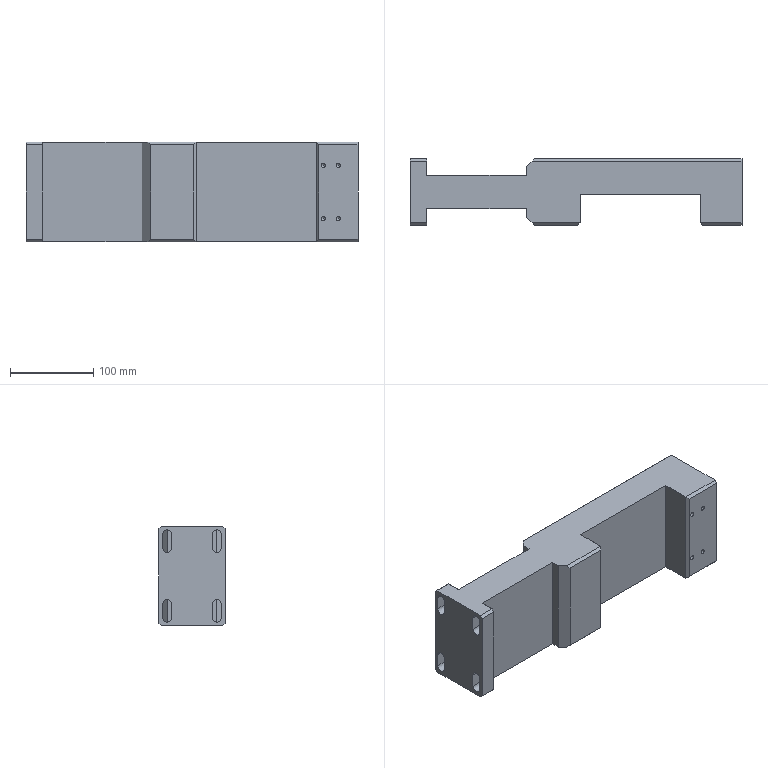Part | 1 solid | 84 faces | box 400 x 80 x 120 mm | volume 2575819 mm3 | plane 52 | cylinder 20 | cone 12 | commonest cylinder face diameters 5 x8 11 x8 6.8 x4